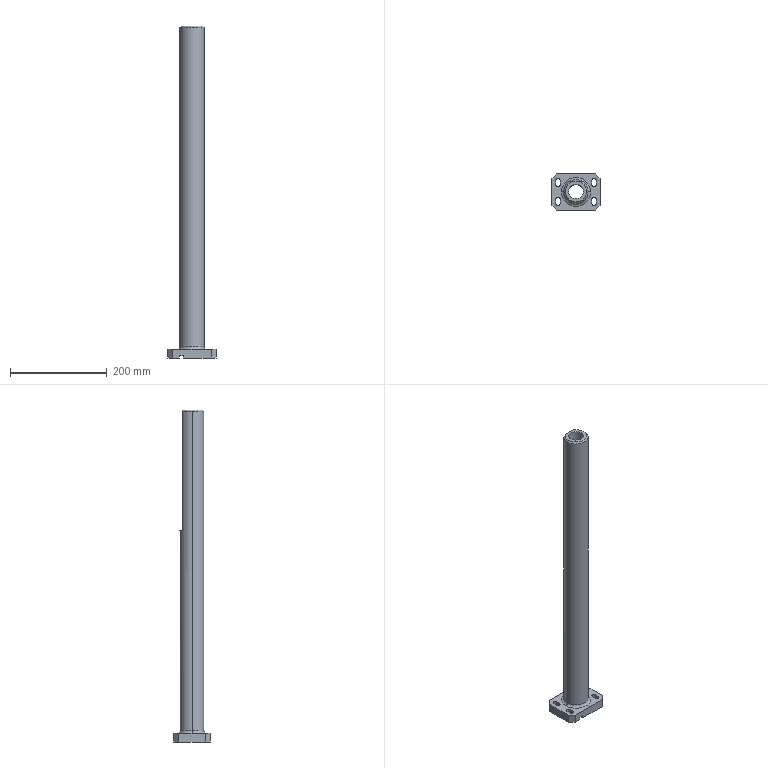Part | STEP file | PN_0024 | 1 solid | 46 faces | box 100 x 75 x 688 mm | volume 922519 mm3 | plane 25 | cylinder 16 | cone 3 | torus 2 | commonest cylinder face diameters 9 x8 3.3 x4 30 x2 50 x2